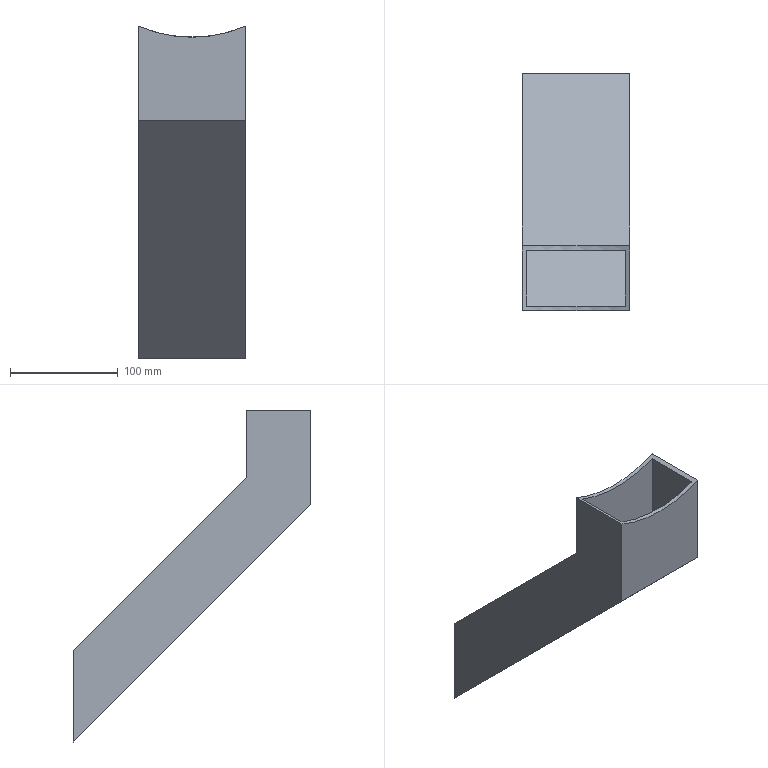Part | NX | features DATUM_CSYS 3, EXTRUDE 2, SKETCH 2, CHAMFER 1, SHELL 1 | 1 solid | 14 faces | box 100 x 220.919 x 308.781 mm | volume 414084 mm3 | plane 13 | cylinder 1 | commonest cylinder face diameters 250 x1
STEP:
#1=CARTESIAN_POINT('',(-50.,30.,75.436));
#2=VERTEX_POINT('',#1);
#3=CARTESIAN_POINT('',(-50.,-30.,75.436));
#4=VERTEX_POINT('',#3);
#5=CARTESIAN_POINT('',(-50.,160.,75.436));
#6=DIRECTION('',(0.,-1.,0.));
#7=VECTOR('',#6,1000.);
#8=LINE('',#5,#7);
#9=EDGE_CURVE('',#2,#4,#8,.T.);
#10=ORIENTED_EDGE('',*,*,#9,.F.);
#11=CARTESIAN_POINT('',(-50.,30.,12.426));
#12=VERTEX_POINT('',#11);
#13=CARTESIAN_POINT('',(-50.,30.,80.));
#14=DIRECTION('',(0.,0.,-1.));
#15=VECTOR('',#14,1000.);
#16=LINE('',#13,#15);
#17=EDGE_CURVE('',#2,#12,#16,.T.);
#18=ORIENTED_EDGE('',*,*,#17,.T.);
#19=CARTESIAN_POINT('',(-50.,190.919,-148.492));
#20=VERTEX_POINT('',#19);
#21=CARTESIAN_POINT('',(-50.,21.213,21.213));
#22=DIRECTION('',(0.,0.7071,-0.7071));
#23=VECTOR('',#22,1000.);
#24=LINE('',#21,#23);
#25=EDGE_CURVE('',#12,#20,#24,.T.);
#26=ORIENTED_EDGE('',*,*,#25,.T.);
#27=CARTESIAN_POINT('',(-50.,190.919,-233.345));
#28=VERTEX_POINT('',#27);
#29=CARTESIAN_POINT('',(-50.,190.919,0.));
#30=DIRECTION('',(0.,0.,-1.));
#31=VECTOR('',#30,1000.);
#32=LINE('',#29,#31);
#33=EDGE_CURVE('',#20,#28,#32,.T.);
#34=ORIENTED_EDGE('',*,*,#33,.T.);
#35=CARTESIAN_POINT('',(-50.,-30.,-12.426));
#36=VERTEX_POINT('',#35);
#37=CARTESIAN_POINT('',(-50.,-21.213,-21.213));
#38=DIRECTION('',(0.,0.7071,-0.7071));
#39=VECTOR('',#38,1000.);
#40=LINE('',#37,#39);
#41=EDGE_CURVE('',#36,#28,#40,.T.);
#42=ORIENTED_EDGE('',*,*,#41,.F.);
#43=CARTESIAN_POINT('',(-50.,-30.,80.));
#44=DIRECTION('',(0.,0.,-1.));
#45=VECTOR('',#44,1000.);
#46=LINE('',#43,#45);
#47=EDGE_CURVE('',#4,#36,#46,.T.);
#48=ORIENTED_EDGE('',*,*,#47,.F.);
#49=EDGE_LOOP('',(#10,#18,#26,#34,#42,#48));
#50=FACE_BOUND('',#49,.T.);
#51=CARTESIAN_POINT('',(-50.,0.,0.));
#52=DIRECTION('',(-1.,0.,0.));
#53=DIRECTION('',(0.,0.7071,-0.7071));
#54=AXIS2_PLACEMENT_3D('',#51,#52,#53);
#55=PLANE('',#54);
#56=ADVANCED_FACE('',(#50),#55,.T.);
#57=CARTESIAN_POINT('',(50.,-30.,75.436));
#58=VERTEX_POINT('',#57);
#59=CARTESIAN_POINT('',(50.,30.,75.436));
#60=VERTEX_POINT('',#59);
#61=CARTESIAN_POINT('',(50.,160.,75.436));
#62=DIRECTION('',(0.,-1.,0.));
#63=VECTOR('',#62,1000.);
#64=LINE('',#61,#63);
#65=EDGE_CURVE('',#58,#60,#64,.F.);
#66=ORIENTED_EDGE('',*,*,#65,.F.);
#67=CARTESIAN_POINT('',(50.,-30.,-12.426));
#68=VERTEX_POINT('',#67);
#69=CARTESIAN_POINT('',(50.,-30.,80.));
#70=DIRECTION('',(0.,0.,-1.));
#71=VECTOR('',#70,1000.);
#72=LINE('',#69,#71);
#73=EDGE_CURVE('',#58,#68,#72,.T.);
#74=ORIENTED_EDGE('',*,*,#73,.T.);
#75=CARTESIAN_POINT('',(50.,190.919,-233.345));
#76=VERTEX_POINT('',#75);
#77=CARTESIAN_POINT('',(50.,-21.213,-21.213));
#78=DIRECTION('',(0.,0.7071,-0.7071));
#79=VECTOR('',#78,1000.);
#80=LINE('',#77,#79);
#81=EDGE_CURVE('',#68,#76,#80,.T.);
#82=ORIENTED_EDGE('',*,*,#81,.T.);
#83=CARTESIAN_POINT('',(50.,190.919,-148.492));
#84=VERTEX_POINT('',#83);
#85=CARTESIAN_POINT('',(50.,190.919,80.));
#86=DIRECTION('',(0.,0.,-1.));
#87=VECTOR('',#86,1000.);
#88=LINE('',#85,#87);
#89=EDGE_CURVE('',#76,#84,#88,.F.);
#90=ORIENTED_EDGE('',*,*,#89,.T.);
#91=CARTESIAN_POINT('',(50.,30.,12.426));
#92=VERTEX_POINT('',#91);
#93=CARTESIAN_POINT('',(50.,21.213,21.213));
#94=DIRECTION('',(0.,0.7071,-0.7071));
#95=VECTOR('',#94,1000.);
#96=LINE('',#93,#95);
#97=EDGE_CURVE('',#92,#84,#96,.T.);
#98=ORIENTED_EDGE('',*,*,#97,.F.);
#99=CARTESIAN_POINT('',(50.,30.,80.));
#100=DIRECTION('',(0.,0.,-1.));
#101=VECTOR('',#100,1000.);
#102=LINE('',#99,#101);
#103=EDGE_CURVE('',#60,#92,#102,.T.);
#104=ORIENTED_EDGE('',*,*,#103,.F.);
#105=EDGE_LOOP('',(#66,#74,#82,#90,#98,#104));
#106=FACE_BOUND('',#105,.T.);
#107=CARTESIAN_POINT('',(50.,0.,80.));
#108=DIRECTION('',(-1.,0.,0.));
#109=DIRECTION('',(0.,0.,-1.));
#110=AXIS2_PLACEMENT_3D('',#107,#108,#109);
#111=PLANE('',#110);
#112=ADVANCED_FACE('',(#106),#111,.F.);
#113=CARTESIAN_POINT('',(0.,-30.,190.));
#114=DIRECTION('',(0.,-1.,0.));
#115=DIRECTION('',(0.,0.,-1.));
#116=AXIS2_PLACEMENT_3D('',#113,#114,#115);
#117=CIRCLE('',#116,125.);
#118=EDGE_CURVE('',#4,#58,#117,.T.);
#119=ORIENTED_EDGE('',*,*,#118,.F.);
#120=ORIENTED_EDGE('',*,*,#47,.T.);
#121=CARTESIAN_POINT('',(-50.,-30.,-12.426));
#122=DIRECTION('',(1.,0.,0.));
#123=VECTOR('',#122,1000.);
#124=LINE('',#121,#123);
#125=EDGE_CURVE('',#36,#68,#124,.T.);
#126=ORIENTED_EDGE('',*,*,#125,.T.);
#127=ORIENTED_EDGE('',*,*,#73,.F.);
#128=EDGE_LOOP('',(#119,#120,#126,#127));
#129=FACE_BOUND('',#128,.T.);
#130=CARTESIAN_POINT('',(-50.,-30.,80.));
#131=DIRECTION('',(0.,-1.,0.));
#132=DIRECTION('',(0.,0.,-1.));
#133=AXIS2_PLACEMENT_3D('',#130,#131,#132);
#134=PLANE('',#133);
#135=ADVANCED_FACE('',(#129),#134,.T.);
#136=ORIENTED_EDGE('',*,*,#81,.F.);
#137=ORIENTED_EDGE('',*,*,#125,.F.);
#138=ORIENTED_EDGE('',*,*,#41,.T.);
#139=CARTESIAN_POINT('',(-50.,190.919,-233.345));
#140=DIRECTION('',(1.,0.,0.));
#141=VECTOR('',#140,1000.);
#142=LINE('',#139,#141);
#143=EDGE_CURVE('',#28,#76,#142,.T.);
#144=ORIENTED_EDGE('',*,*,#143,.T.);
#145=EDGE_LOOP('',(#136,#137,#138,#144));
#146=FACE_BOUND('',#145,.T.);
#147=CARTESIAN_POINT('',(-50.,-21.213,-21.213));
#148=DIRECTION('',(0.,-0.7071,-0.7071));
#149=DIRECTION('',(0.,0.7071,-0.7071));
#150=AXIS2_PLACEMENT_3D('',#147,#148,#149);
#151=PLANE('',#150);
#152=ADVANCED_FACE('',(#146),#151,.T.);
#153=ORIENTED_EDGE('',*,*,#17,.F.);
#154=CARTESIAN_POINT('',(0.,30.,190.));
#155=DIRECTION('',(0.,-1.,0.));
#156=DIRECTION('',(0.,0.,-1.));
#157=AXIS2_PLACEMENT_3D('',#154,#155,#156);
#158=CIRCLE('',#157,125.);
#159=EDGE_CURVE('',#2,#60,#158,.T.);
#160=ORIENTED_EDGE('',*,*,#159,.T.);
#161=ORIENTED_EDGE('',*,*,#103,.T.);
#162=CARTESIAN_POINT('',(-50.,30.,12.426));
#163=DIRECTION('',(1.,0.,0.));
#164=VECTOR('',#163,1000.);
#165=LINE('',#162,#164);
#166=EDGE_CURVE('',#12,#92,#165,.T.);
#167=ORIENTED_EDGE('',*,*,#166,.F.);
#168=EDGE_LOOP('',(#153,#160,#161,#167));
#169=FACE_BOUND('',#168,.T.);
#170=CARTESIAN_POINT('',(-50.,30.,80.));
#171=DIRECTION('',(0.,-1.,0.));
#172=DIRECTION('',(0.,0.,-1.));
#173=AXIS2_PLACEMENT_3D('',#170,#171,#172);
#174=PLANE('',#173);
#175=ADVANCED_FACE('',(#169),#174,.F.);
#176=ORIENTED_EDGE('',*,*,#97,.T.);
#177=CARTESIAN_POINT('',(-50.,190.919,-148.492));
#178=DIRECTION('',(-1.,0.,0.));
#179=VECTOR('',#178,1000.);
#180=LINE('',#177,#179);
#181=EDGE_CURVE('',#84,#20,#180,.T.);
#182=ORIENTED_EDGE('',*,*,#181,.T.);
#183=ORIENTED_EDGE('',*,*,#25,.F.);
#184=ORIENTED_EDGE('',*,*,#166,.T.);
#185=EDGE_LOOP('',(#176,#182,#183,#184));
#186=FACE_BOUND('',#185,.T.);
#187=CARTESIAN_POINT('',(-50.,21.213,21.213));
#188=DIRECTION('',(0.,-0.7071,-0.7071));
#189=DIRECTION('',(0.,0.7071,-0.7071));
#190=AXIS2_PLACEMENT_3D('',#187,#188,#189);
#191=PLANE('',#190);
#192=ADVANCED_FACE('',(#186),#191,.F.);
#193=CARTESIAN_POINT('',(-46.,26.,73.772));
#194=VERTEX_POINT('',#193);
#195=CARTESIAN_POINT('',(-46.,26.,10.77));
#196=VERTEX_POINT('',#195);
#197=CARTESIAN_POINT('',(-46.,26.,80.));
#198=DIRECTION('',(0.,0.,-1.));
#199=VECTOR('',#198,1000.);
#200=LINE('',#197,#199);
#201=EDGE_CURVE('',#194,#196,#200,.T.);
#202=ORIENTED_EDGE('',*,*,#201,.F.);
#203=CARTESIAN_POINT('',(-46.,-26.,73.772));
#204=VERTEX_POINT('',#203);
#205=CARTESIAN_POINT('',(-46.,160.,73.772));
#206=DIRECTION('',(0.,-1.,0.));
#207=VECTOR('',#206,1000.);
#208=LINE('',#205,#207);
#209=EDGE_CURVE('',#194,#204,#208,.T.);
#210=ORIENTED_EDGE('',*,*,#209,.T.);
#211=CARTESIAN_POINT('',(-46.,-26.,-10.77));
#212=VERTEX_POINT('',#211);
#213=CARTESIAN_POINT('',(-46.,-26.,80.));
#214=DIRECTION('',(0.,0.,-1.));
#215=VECTOR('',#214,1000.);
#216=LINE('',#213,#215);
#217=EDGE_CURVE('',#204,#212,#216,.T.);
#218=ORIENTED_EDGE('',*,*,#217,.T.);
#219=CARTESIAN_POINT('',(-46.,190.919,-227.688));
#220=VERTEX_POINT('',#219);
#221=CARTESIAN_POINT('',(-46.,-18.385,-18.385));
#222=DIRECTION('',(0.,0.7071,-0.7071));
#223=VECTOR('',#222,1000.);
#224=LINE('',#221,#223);
#225=EDGE_CURVE('',#212,#220,#224,.T.);
#226=ORIENTED_EDGE('',*,*,#225,.T.);
#227=CARTESIAN_POINT('',(-46.,190.919,-154.149));
#228=VERTEX_POINT('',#227);
#229=CARTESIAN_POINT('',(-46.,190.919,0.));
#230=DIRECTION('',(0.,0.,-1.));
#231=VECTOR('',#230,1000.);
#232=LINE('',#229,#231);
#233=EDGE_CURVE('',#228,#220,#232,.T.);
#234=ORIENTED_EDGE('',*,*,#233,.F.);
#235=CARTESIAN_POINT('',(-46.,18.385,18.385));
#236=DIRECTION('',(0.,0.7071,-0.7071));
#237=VECTOR('',#236,1000.);
#238=LINE('',#235,#237);
#239=EDGE_CURVE('',#196,#228,#238,.T.);
#240=ORIENTED_EDGE('',*,*,#239,.F.);
#241=EDGE_LOOP('',(#202,#210,#218,#226,#234,#240));
#242=FACE_BOUND('',#241,.T.);
#243=CARTESIAN_POINT('',(-46.,0.,0.));
#244=DIRECTION('',(-1.,0.,0.));
#245=DIRECTION('',(0.,0.7071,-0.7071));
#246=AXIS2_PLACEMENT_3D('',#243,#244,#245);
#247=PLANE('',#246);
#248=ADVANCED_FACE('',(#242),#247,.F.);
#249=CARTESIAN_POINT('',(46.,-26.,73.772));
#250=VERTEX_POINT('',#249);
#251=CARTESIAN_POINT('',(46.,-26.,-10.77));
#252=VERTEX_POINT('',#251);
#253=CARTESIAN_POINT('',(46.,-26.,80.));
#254=DIRECTION('',(0.,0.,1.));
#255=VECTOR('',#254,1000.);
#256=LINE('',#253,#255);
#257=EDGE_CURVE('',#250,#252,#256,.F.);
#258=ORIENTED_EDGE('',*,*,#257,.F.);
#259=CARTESIAN_POINT('',(46.,26.,73.772));
#260=VERTEX_POINT('',#259);
#261=CARTESIAN_POINT('',(46.,160.,73.772));
#262=DIRECTION('',(0.,-1.,0.));
#263=VECTOR('',#262,1000.);
#264=LINE('',#261,#263);
#265=EDGE_CURVE('',#250,#260,#264,.F.);
#266=ORIENTED_EDGE('',*,*,#265,.T.);
#267=CARTESIAN_POINT('',(46.,26.,10.77));
#268=VERTEX_POINT('',#267);
#269=CARTESIAN_POINT('',(46.,26.,80.));
#270=DIRECTION('',(0.,0.,1.));
#271=VECTOR('',#270,1000.);
#272=LINE('',#269,#271);
#273=EDGE_CURVE('',#260,#268,#272,.F.);
#274=ORIENTED_EDGE('',*,*,#273,.T.);
#275=CARTESIAN_POINT('',(46.,190.919,-154.149));
#276=VERTEX_POINT('',#275);
#277=CARTESIAN_POINT('',(46.,-21.615,58.385));
#278=DIRECTION('',(0.,-0.7071,0.7071));
#279=VECTOR('',#278,1000.);
#280=LINE('',#277,#279);
#281=EDGE_CURVE('',#268,#276,#280,.F.);
#282=ORIENTED_EDGE('',*,*,#281,.T.);
#283=CARTESIAN_POINT('',(46.,190.919,-227.688));
#284=VERTEX_POINT('',#283);
#285=CARTESIAN_POINT('',(46.,190.919,-233.345));
#286=DIRECTION('',(0.,0.,1.));
#287=VECTOR('',#286,1000.);
#288=LINE('',#285,#287);
#289=EDGE_CURVE('',#276,#284,#288,.F.);
#290=ORIENTED_EDGE('',*,*,#289,.T.);
#291=CARTESIAN_POINT('',(46.,-58.385,21.615));
#292=DIRECTION('',(0.,-0.7071,0.7071));
#293=VECTOR('',#292,1000.);
#294=LINE('',#291,#293);
#295=EDGE_CURVE('',#252,#284,#294,.F.);
#296=ORIENTED_EDGE('',*,*,#295,.F.);
#297=EDGE_LOOP('',(#258,#266,#274,#282,#290,#296));
#298=FACE_BOUND('',#297,.T.);
#299=CARTESIAN_POINT('',(46.,0.,80.));
#300=DIRECTION('',(-1.,0.,0.));
#301=DIRECTION('',(0.,0.,-1.));
#302=AXIS2_PLACEMENT_3D('',#299,#300,#301);
#303=PLANE('',#302);
#304=ADVANCED_FACE('',(#298),#303,.T.);
#305=ORIENTED_EDGE('',*,*,#217,.F.);
#306=CARTESIAN_POINT('',(0.,-26.,190.));
#307=DIRECTION('',(0.,-1.,0.));
#308=DIRECTION('',(0.,0.,-1.));
#309=AXIS2_PLACEMENT_3D('',#306,#307,#308);
#310=CIRCLE('',#309,125.);
#311=EDGE_CURVE('',#204,#250,#310,.T.);
#312=ORIENTED_EDGE('',*,*,#311,.T.);
#313=ORIENTED_EDGE('',*,*,#257,.T.);
#314=CARTESIAN_POINT('',(-50.,-26.,-10.77));
#315=DIRECTION('',(1.,0.,0.));
#316=VECTOR('',#315,1000.);
#317=LINE('',#314,#316);
#318=EDGE_CURVE('',#212,#252,#317,.T.);
#319=ORIENTED_EDGE('',*,*,#318,.F.);
#320=EDGE_LOOP('',(#305,#312,#313,#319));
#321=FACE_BOUND('',#320,.T.);
#322=CARTESIAN_POINT('',(-50.,-26.,80.));
#323=DIRECTION('',(0.,-1.,0.));
#324=DIRECTION('',(0.,0.,-1.));
#325=AXIS2_PLACEMENT_3D('',#322,#323,#324);
#326=PLANE('',#325);
#327=ADVANCED_FACE('',(#321),#326,.F.);
#328=ORIENTED_EDGE('',*,*,#295,.T.);
#329=CARTESIAN_POINT('',(-50.,190.919,-227.688));
#330=DIRECTION('',(1.,0.,0.));
#331=VECTOR('',#330,1000.);
#332=LINE('',#329,#331);
#333=EDGE_CURVE('',#220,#284,#332,.T.);
#334=ORIENTED_EDGE('',*,*,#333,.F.);
#335=ORIENTED_EDGE('',*,*,#225,.F.);
#336=ORIENTED_EDGE('',*,*,#318,.T.);
#337=EDGE_LOOP('',(#328,#334,#335,#336));
#338=FACE_BOUND('',#337,.T.);
#339=CARTESIAN_POINT('',(-50.,-18.385,-18.385));
#340=DIRECTION('',(0.,-0.7071,-0.7071));
#341=DIRECTION('',(0.,0.7071,-0.7071));
#342=AXIS2_PLACEMENT_3D('',#339,#340,#341);
#343=PLANE('',#342);
#344=ADVANCED_FACE('',(#338),#343,.F.);
#345=CARTESIAN_POINT('',(0.,26.,190.));
#346=DIRECTION('',(0.,-1.,0.));
#347=DIRECTION('',(0.,0.,-1.));
#348=AXIS2_PLACEMENT_3D('',#345,#346,#347);
#349=CIRCLE('',#348,125.);
#350=EDGE_CURVE('',#194,#260,#349,.T.);
#351=ORIENTED_EDGE('',*,*,#350,.F.);
#352=ORIENTED_EDGE('',*,*,#201,.T.);
#353=CARTESIAN_POINT('',(-50.,26.,10.77));
#354=DIRECTION('',(1.,0.,0.));
#355=VECTOR('',#354,1000.);
#356=LINE('',#353,#355);
#357=EDGE_CURVE('',#196,#268,#356,.T.);
#358=ORIENTED_EDGE('',*,*,#357,.T.);
#359=ORIENTED_EDGE('',*,*,#273,.F.);
#360=EDGE_LOOP('',(#351,#352,#358,#359));
#361=FACE_BOUND('',#360,.T.);
#362=CARTESIAN_POINT('',(-50.,26.,80.));
#363=DIRECTION('',(0.,-1.,0.));
#364=DIRECTION('',(0.,0.,-1.));
#365=AXIS2_PLACEMENT_3D('',#362,#363,#364);
#366=PLANE('',#365);
#367=ADVANCED_FACE('',(#361),#366,.T.);
#368=ORIENTED_EDGE('',*,*,#281,.F.);
#369=ORIENTED_EDGE('',*,*,#357,.F.);
#370=ORIENTED_EDGE('',*,*,#239,.T.);
#371=CARTESIAN_POINT('',(-50.,190.919,-154.149));
#372=DIRECTION('',(1.,0.,0.));
#373=VECTOR('',#372,1000.);
#374=LINE('',#371,#373);
#375=EDGE_CURVE('',#228,#276,#374,.T.);
#376=ORIENTED_EDGE('',*,*,#375,.T.);
#377=EDGE_LOOP('',(#368,#369,#370,#376));
#378=FACE_BOUND('',#377,.T.);
#379=CARTESIAN_POINT('',(-50.,18.385,18.385));
#380=DIRECTION('',(0.,-0.7071,-0.7071));
#381=DIRECTION('',(0.,0.7071,-0.7071));
#382=AXIS2_PLACEMENT_3D('',#379,#380,#381);
#383=PLANE('',#382);
#384=ADVANCED_FACE('',(#378),#383,.T.);
#385=ORIENTED_EDGE('',*,*,#33,.F.);
#386=ORIENTED_EDGE('',*,*,#181,.F.);
#387=ORIENTED_EDGE('',*,*,#89,.F.);
#388=ORIENTED_EDGE('',*,*,#143,.F.);
#389=EDGE_LOOP('',(#385,#386,#387,#388));
#390=FACE_BOUND('',#389,.T.);
#391=ORIENTED_EDGE('',*,*,#375,.F.);
#392=ORIENTED_EDGE('',*,*,#233,.T.);
#393=ORIENTED_EDGE('',*,*,#333,.T.);
#394=ORIENTED_EDGE('',*,*,#289,.F.);
#395=EDGE_LOOP('',(#391,#392,#393,#394));
#396=FACE_BOUND('',#395,.T.);
#397=CARTESIAN_POINT('',(-50.,190.919,-233.345));
#398=DIRECTION('',(0.,1.,0.));
#399=DIRECTION('',(-1.,0.,0.));
#400=AXIS2_PLACEMENT_3D('',#397,#398,#399);
#401=PLANE('',#400);
#402=ADVANCED_FACE('',(#390,#396),#401,.T.);
#403=ORIENTED_EDGE('',*,*,#118,.T.);
#404=ORIENTED_EDGE('',*,*,#65,.T.);
#405=ORIENTED_EDGE('',*,*,#159,.F.);
#406=ORIENTED_EDGE('',*,*,#9,.T.);
#407=EDGE_LOOP('',(#403,#404,#405,#406));
#408=FACE_BOUND('',#407,.T.);
#409=ORIENTED_EDGE('',*,*,#209,.F.);
#410=ORIENTED_EDGE('',*,*,#350,.T.);
#411=ORIENTED_EDGE('',*,*,#265,.F.);
#412=ORIENTED_EDGE('',*,*,#311,.F.);
#413=EDGE_LOOP('',(#409,#410,#411,#412));
#414=FACE_BOUND('',#413,.T.);
#415=CARTESIAN_POINT('',(0.,160.,190.));
#416=DIRECTION('',(0.,-1.,0.));
#417=DIRECTION('',(0.,0.,-1.));
#418=AXIS2_PLACEMENT_3D('',#415,#416,#417);
#419=CYLINDRICAL_SURFACE('',#418,125.);
#420=ADVANCED_FACE('',(#408,#414),#419,.F.);
#421=CLOSED_SHELL('',(#56,#112,#135,#152,#175,#192,#248,#304,#327,#344,#367,#384,#402,#420));
#422=MANIFOLD_SOLID_BREP('',#421);
#423=(LENGTH_UNIT()NAMED_UNIT(*)SI_UNIT(.MILLI.,.METRE.));
#424=UNCERTAINTY_MEASURE_WITH_UNIT(LENGTH_MEASURE(0.00001),#423,'','');
#425=(NAMED_UNIT(*)PLANE_ANGLE_UNIT()SI_UNIT($,.RADIAN.));
#426=(NAMED_UNIT(*)SI_UNIT($,.STERADIAN.)SOLID_ANGLE_UNIT());
#427=(GEOMETRIC_REPRESENTATION_CONTEXT(3)GLOBAL_UNCERTAINTY_ASSIGNED_CONTEXT((#424))GLOBAL_UNIT_ASSIGNED_CONTEXT((#423,#425,#426))REPRESENTATION_CONTEXT('',''));
#428=ADVANCED_BREP_SHAPE_REPRESENTATION('',(#422),#427);